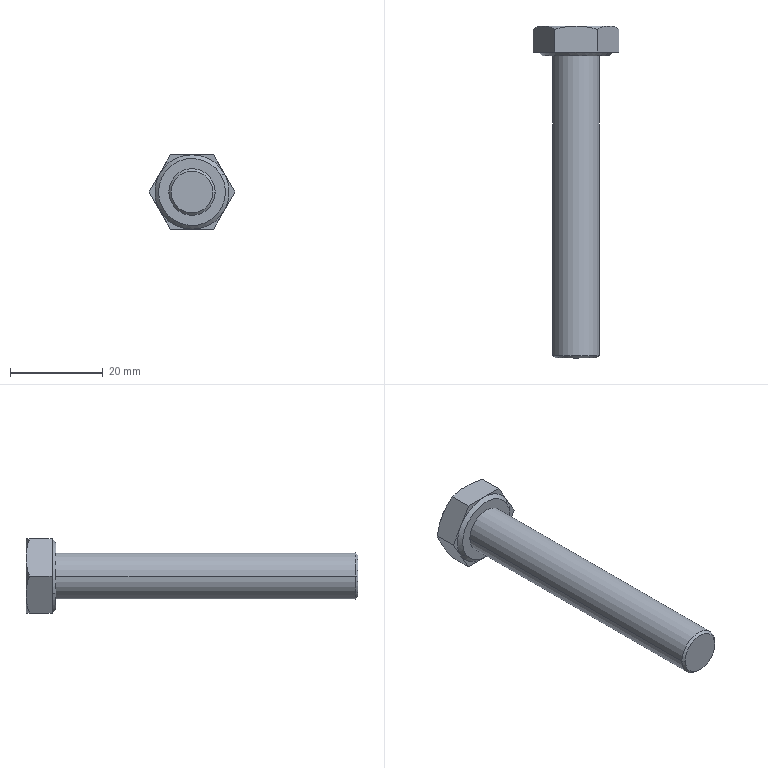Part | STEP file | SOLID | 1 solid | 27 faces | box 18.475 x 71.4 x 16 mm | volume 6484 mm3 | plane 15 | cone 10 | cylinder 2 | commonest cylinder face diameters 10 x2